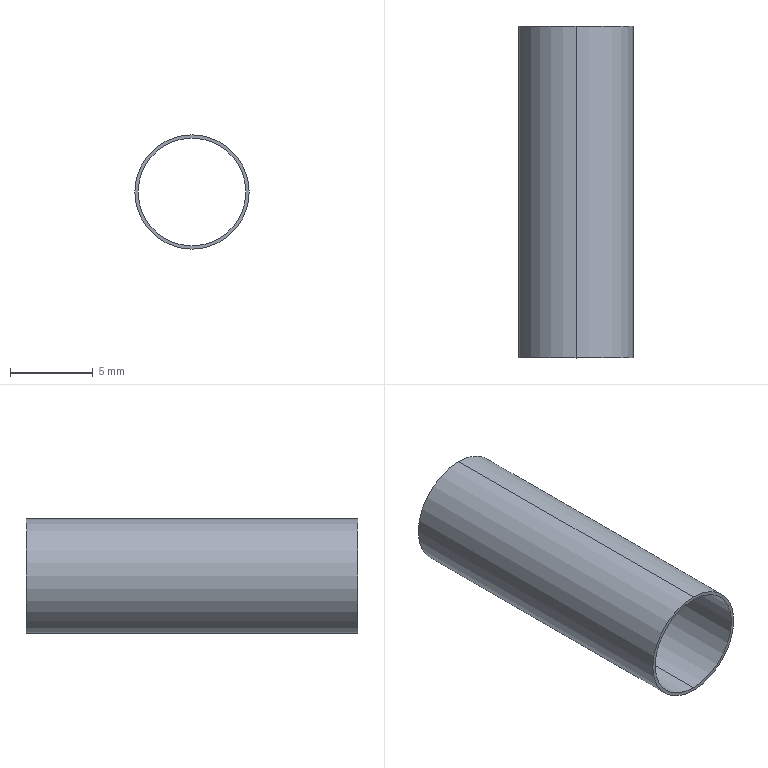Part | SolidWorks | features ExtruThin 1 | 1 solid | 6 faces | box 6.9 x 20 x 6.9 mm | volume 84.195 mm3 | cylinder 4 | plane 2 | commonest cylinder face diameters 6.5 x2 6.9 x2
STEP:
#1=CARTESIAN_POINT('',(0.,20.,-3.25));
#2=VERTEX_POINT('',#1);
#3=CARTESIAN_POINT('',(0.,20.,3.25));
#4=VERTEX_POINT('',#3);
#5=CARTESIAN_POINT('',(0.,20.,0.));
#6=DIRECTION('',(0.,1.,0.));
#7=DIRECTION('',(0.,0.,1.));
#8=AXIS2_PLACEMENT_3D('',#5,#6,#7);
#9=CIRCLE('',#8,3.25);
#10=EDGE_CURVE('',#2,#4,#9,.T.);
#11=ORIENTED_EDGE('',*,*,#10,.T.);
#12=CARTESIAN_POINT('',(0.,0.,3.25));
#13=VERTEX_POINT('',#12);
#14=CARTESIAN_POINT('',(0.,20.,3.25));
#15=DIRECTION('',(0.,-1.,0.));
#16=VECTOR('',#15,1000.);
#17=LINE('',#14,#16);
#18=EDGE_CURVE('',#4,#13,#17,.T.);
#19=ORIENTED_EDGE('',*,*,#18,.T.);
#20=CARTESIAN_POINT('',(0.,0.,-3.25));
#21=VERTEX_POINT('',#20);
#22=CARTESIAN_POINT('',(0.,0.,0.));
#23=DIRECTION('',(0.,1.,0.));
#24=DIRECTION('',(0.,0.,1.));
#25=AXIS2_PLACEMENT_3D('',#22,#23,#24);
#26=CIRCLE('',#25,3.25);
#27=EDGE_CURVE('',#21,#13,#26,.T.);
#28=ORIENTED_EDGE('',*,*,#27,.F.);
#29=CARTESIAN_POINT('',(0.,20.,-3.25));
#30=DIRECTION('',(0.,-1.,0.));
#31=VECTOR('',#30,1000.);
#32=LINE('',#29,#31);
#33=EDGE_CURVE('',#2,#21,#32,.T.);
#34=ORIENTED_EDGE('',*,*,#33,.F.);
#35=EDGE_LOOP('',(#11,#19,#28,#34));
#36=FACE_OUTER_BOUND('',#35,.T.);
#37=CARTESIAN_POINT('',(0.,20.,0.));
#38=DIRECTION('',(0.,-1.,0.));
#39=DIRECTION('',(0.,0.,-1.));
#40=AXIS2_PLACEMENT_3D('',#37,#38,#39);
#41=CYLINDRICAL_SURFACE('',#40,3.25);
#42=ADVANCED_FACE('',(#36),#41,.F.);
#43=CARTESIAN_POINT('',(0.,20.,3.45));
#44=VERTEX_POINT('',#43);
#45=CARTESIAN_POINT('',(0.,20.,-3.45));
#46=VERTEX_POINT('',#45);
#47=CARTESIAN_POINT('',(0.,20.,0.));
#48=DIRECTION('',(0.,1.,0.));
#49=DIRECTION('',(1.,0.,0.));
#50=AXIS2_PLACEMENT_3D('',#47,#48,#49);
#51=CIRCLE('',#50,3.45);
#52=EDGE_CURVE('',#44,#46,#51,.T.);
#53=ORIENTED_EDGE('',*,*,#52,.F.);
#54=CARTESIAN_POINT('',(0.,0.,3.45));
#55=VERTEX_POINT('',#54);
#56=CARTESIAN_POINT('',(0.,20.,3.45));
#57=DIRECTION('',(0.,-1.,0.));
#58=VECTOR('',#57,1000.);
#59=LINE('',#56,#58);
#60=EDGE_CURVE('',#44,#55,#59,.T.);
#61=ORIENTED_EDGE('',*,*,#60,.T.);
#62=CARTESIAN_POINT('',(0.,0.,-3.45));
#63=VERTEX_POINT('',#62);
#64=CARTESIAN_POINT('',(0.,0.,0.));
#65=DIRECTION('',(0.,1.,0.));
#66=DIRECTION('',(1.,0.,0.));
#67=AXIS2_PLACEMENT_3D('',#64,#65,#66);
#68=CIRCLE('',#67,3.45);
#69=EDGE_CURVE('',#55,#63,#68,.T.);
#70=ORIENTED_EDGE('',*,*,#69,.T.);
#71=CARTESIAN_POINT('',(0.,20.,-3.45));
#72=DIRECTION('',(0.,-1.,0.));
#73=VECTOR('',#72,1000.);
#74=LINE('',#71,#73);
#75=EDGE_CURVE('',#46,#63,#74,.T.);
#76=ORIENTED_EDGE('',*,*,#75,.F.);
#77=EDGE_LOOP('',(#53,#61,#70,#76));
#78=FACE_OUTER_BOUND('',#77,.T.);
#79=CARTESIAN_POINT('',(0.,20.,0.));
#80=DIRECTION('',(0.,-1.,0.));
#81=DIRECTION('',(0.,0.,-1.));
#82=AXIS2_PLACEMENT_3D('',#79,#80,#81);
#83=CYLINDRICAL_SURFACE('',#82,3.45);
#84=ADVANCED_FACE('',(#78),#83,.T.);
#85=CARTESIAN_POINT('',(0.,20.,0.));
#86=DIRECTION('',(0.,1.,0.));
#87=DIRECTION('',(1.,0.,0.));
#88=AXIS2_PLACEMENT_3D('',#85,#86,#87);
#89=CIRCLE('',#88,3.45);
#90=EDGE_CURVE('',#46,#44,#89,.T.);
#91=ORIENTED_EDGE('',*,*,#90,.T.);
#92=ORIENTED_EDGE('',*,*,#52,.T.);
#93=EDGE_LOOP('',(#91,#92));
#94=FACE_OUTER_BOUND('',#93,.T.);
#95=ORIENTED_EDGE('',*,*,#10,.F.);
#96=CARTESIAN_POINT('',(0.,20.,0.));
#97=DIRECTION('',(0.,1.,0.));
#98=DIRECTION('',(0.,0.,1.));
#99=AXIS2_PLACEMENT_3D('',#96,#97,#98);
#100=CIRCLE('',#99,3.25);
#101=EDGE_CURVE('',#4,#2,#100,.T.);
#102=ORIENTED_EDGE('',*,*,#101,.F.);
#103=EDGE_LOOP('',(#95,#102));
#104=FACE_BOUND('',#103,.T.);
#105=CARTESIAN_POINT('',(0.,20.,0.));
#106=DIRECTION('',(0.,1.,0.));
#107=DIRECTION('',(0.,0.,1.));
#108=AXIS2_PLACEMENT_3D('',#105,#106,#107);
#109=PLANE('',#108);
#110=ADVANCED_FACE('',(#94,#104),#109,.T.);
#111=CARTESIAN_POINT('',(0.,0.,0.));
#112=DIRECTION('',(0.,1.,0.));
#113=DIRECTION('',(1.,0.,0.));
#114=AXIS2_PLACEMENT_3D('',#111,#112,#113);
#115=CIRCLE('',#114,3.45);
#116=EDGE_CURVE('',#63,#55,#115,.T.);
#117=ORIENTED_EDGE('',*,*,#116,.F.);
#118=ORIENTED_EDGE('',*,*,#69,.F.);
#119=EDGE_LOOP('',(#117,#118));
#120=FACE_OUTER_BOUND('',#119,.T.);
#121=ORIENTED_EDGE('',*,*,#27,.T.);
#122=CARTESIAN_POINT('',(0.,0.,0.));
#123=DIRECTION('',(0.,1.,0.));
#124=DIRECTION('',(0.,0.,1.));
#125=AXIS2_PLACEMENT_3D('',#122,#123,#124);
#126=CIRCLE('',#125,3.25);
#127=EDGE_CURVE('',#13,#21,#126,.T.);
#128=ORIENTED_EDGE('',*,*,#127,.T.);
#129=EDGE_LOOP('',(#121,#128));
#130=FACE_BOUND('',#129,.T.);
#131=CARTESIAN_POINT('',(0.,0.,0.));
#132=DIRECTION('',(0.,1.,0.));
#133=DIRECTION('',(0.,0.,1.));
#134=AXIS2_PLACEMENT_3D('',#131,#132,#133);
#135=PLANE('',#134);
#136=ADVANCED_FACE('',(#120,#130),#135,.F.);
#137=ORIENTED_EDGE('',*,*,#60,.F.);
#138=ORIENTED_EDGE('',*,*,#90,.F.);
#139=ORIENTED_EDGE('',*,*,#75,.T.);
#140=ORIENTED_EDGE('',*,*,#116,.T.);
#141=EDGE_LOOP('',(#137,#138,#139,#140));
#142=FACE_OUTER_BOUND('',#141,.T.);
#143=CARTESIAN_POINT('',(0.,20.,0.));
#144=DIRECTION('',(0.,-1.,0.));
#145=DIRECTION('',(0.,0.,-1.));
#146=AXIS2_PLACEMENT_3D('',#143,#144,#145);
#147=CYLINDRICAL_SURFACE('',#146,3.45);
#148=ADVANCED_FACE('',(#142),#147,.T.);
#149=ORIENTED_EDGE('',*,*,#18,.F.);
#150=ORIENTED_EDGE('',*,*,#101,.T.);
#151=ORIENTED_EDGE('',*,*,#33,.T.);
#152=ORIENTED_EDGE('',*,*,#127,.F.);
#153=EDGE_LOOP('',(#149,#150,#151,#152));
#154=FACE_OUTER_BOUND('',#153,.T.);
#155=CARTESIAN_POINT('',(0.,20.,0.));
#156=DIRECTION('',(0.,-1.,0.));
#157=DIRECTION('',(0.,0.,-1.));
#158=AXIS2_PLACEMENT_3D('',#155,#156,#157);
#159=CYLINDRICAL_SURFACE('',#158,3.25);
#160=ADVANCED_FACE('',(#154),#159,.F.);
#161=CLOSED_SHELL('',(#42,#84,#110,#136,#148,#160));
#162=MANIFOLD_SOLID_BREP('',#161);
#163=CARTESIAN_POINT('',(0.,0.,0.));
#164=DIRECTION('',(0.,0.,1.));
#165=DIRECTION('',(1.,0.,0.));
#166=AXIS2_PLACEMENT_3D('',#163,#164,#165);
#167=(LENGTH_UNIT()NAMED_UNIT(*)SI_UNIT(.MILLI.,.METRE.));
#168=UNCERTAINTY_MEASURE_WITH_UNIT(LENGTH_MEASURE(0.00001),#167,'','');
#169=(NAMED_UNIT(*)PLANE_ANGLE_UNIT()SI_UNIT($,.RADIAN.));
#170=(NAMED_UNIT(*)SI_UNIT($,.STERADIAN.)SOLID_ANGLE_UNIT());
#171=(GEOMETRIC_REPRESENTATION_CONTEXT(3)GLOBAL_UNCERTAINTY_ASSIGNED_CONTEXT((#168))GLOBAL_UNIT_ASSIGNED_CONTEXT((#167,#169,#170))REPRESENTATION_CONTEXT('',''));
#172=ADVANCED_BREP_SHAPE_REPRESENTATION('',(#162,#166),#171);